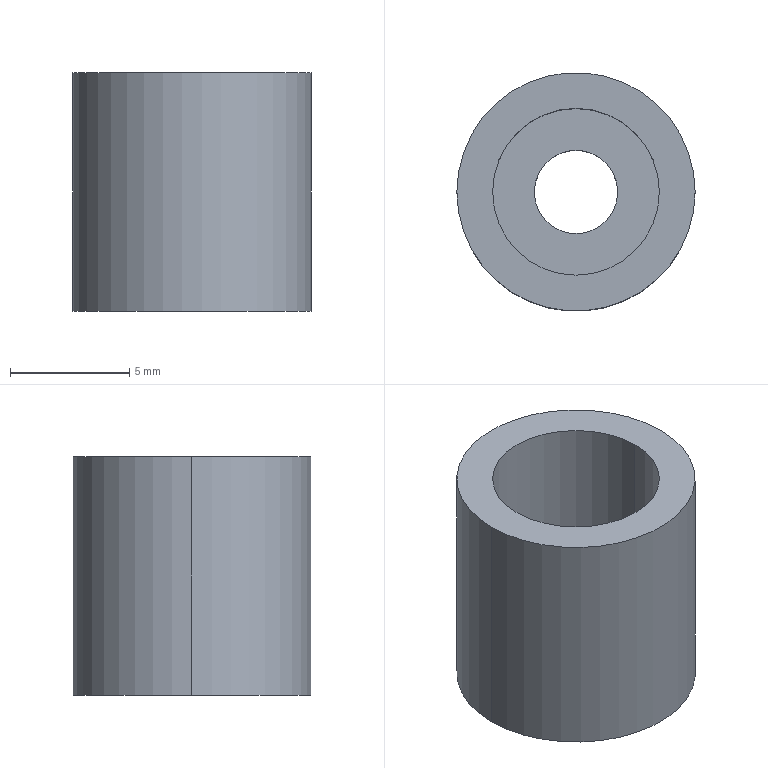Part | NX | features BREP 1 | 1 solid | 9 faces | box 10 x 10 x 10 mm | volume 544.87 mm3 | cylinder 6 | plane 3 | commonest cylinder face diameters 3.5 x2 7 x2 10 x2
STEP:
#1=CARTESIAN_POINT('',(-3.5,0.,10.));
#2=VERTEX_POINT('',#1);
#3=CARTESIAN_POINT('',(-3.5,0.,5.));
#4=VERTEX_POINT('',#3);
#5=CARTESIAN_POINT('',(-3.5,0.,10.));
#6=DIRECTION('',(0.,0.,1.));
#7=VECTOR('',#6,1000.);
#8=LINE('',#5,#7);
#9=EDGE_CURVE('',#2,#4,#8,.F.);
#10=ORIENTED_EDGE('',*,*,#9,.T.);
#11=CARTESIAN_POINT('',(3.5,0.,5.));
#12=VERTEX_POINT('',#11);
#13=CARTESIAN_POINT('',(0.,0.,5.));
#14=DIRECTION('',(0.,0.,1.));
#15=DIRECTION('',(1.,0.,0.));
#16=AXIS2_PLACEMENT_3D('',#13,#14,#15);
#17=CIRCLE('',#16,3.5);
#18=EDGE_CURVE('',#12,#4,#17,.T.);
#19=ORIENTED_EDGE('',*,*,#18,.F.);
#20=CARTESIAN_POINT('',(3.5,0.,10.));
#21=VERTEX_POINT('',#20);
#22=CARTESIAN_POINT('',(3.5,0.,10.));
#23=DIRECTION('',(0.,0.,1.));
#24=VECTOR('',#23,1000.);
#25=LINE('',#22,#24);
#26=EDGE_CURVE('',#21,#12,#25,.F.);
#27=ORIENTED_EDGE('',*,*,#26,.F.);
#28=CARTESIAN_POINT('',(0.,0.,10.));
#29=DIRECTION('',(0.,0.,1.));
#30=DIRECTION('',(1.,0.,0.));
#31=AXIS2_PLACEMENT_3D('',#28,#29,#30);
#32=CIRCLE('',#31,3.5);
#33=EDGE_CURVE('',#21,#2,#32,.T.);
#34=ORIENTED_EDGE('',*,*,#33,.T.);
#35=EDGE_LOOP('',(#10,#19,#27,#34));
#36=FACE_BOUND('',#35,.T.);
#37=CARTESIAN_POINT('',(0.,0.,10.));
#38=DIRECTION('',(0.,0.,1.));
#39=DIRECTION('',(1.,0.,0.));
#40=AXIS2_PLACEMENT_3D('',#37,#38,#39);
#41=CYLINDRICAL_SURFACE('',#40,3.5);
#42=ADVANCED_FACE('',(#36),#41,.F.);
#43=ORIENTED_EDGE('',*,*,#18,.T.);
#44=CARTESIAN_POINT('',(0.,0.,5.));
#45=DIRECTION('',(0.,0.,1.));
#46=DIRECTION('',(1.,0.,0.));
#47=AXIS2_PLACEMENT_3D('',#44,#45,#46);
#48=CIRCLE('',#47,3.5);
#49=EDGE_CURVE('',#4,#12,#48,.T.);
#50=ORIENTED_EDGE('',*,*,#49,.T.);
#51=EDGE_LOOP('',(#43,#50));
#52=FACE_BOUND('',#51,.T.);
#53=CARTESIAN_POINT('',(1.75,0.,5.));
#54=VERTEX_POINT('',#53);
#55=CARTESIAN_POINT('',(-1.75,0.,5.));
#56=VERTEX_POINT('',#55);
#57=CARTESIAN_POINT('',(0.,0.,5.));
#58=DIRECTION('',(0.,0.,1.));
#59=DIRECTION('',(1.,0.,0.));
#60=AXIS2_PLACEMENT_3D('',#57,#58,#59);
#61=CIRCLE('',#60,1.75);
#62=EDGE_CURVE('',#54,#56,#61,.T.);
#63=ORIENTED_EDGE('',*,*,#62,.F.);
#64=CARTESIAN_POINT('',(0.,0.,5.));
#65=DIRECTION('',(0.,0.,1.));
#66=DIRECTION('',(1.,0.,0.));
#67=AXIS2_PLACEMENT_3D('',#64,#65,#66);
#68=CIRCLE('',#67,1.75);
#69=EDGE_CURVE('',#56,#54,#68,.T.);
#70=ORIENTED_EDGE('',*,*,#69,.F.);
#71=EDGE_LOOP('',(#63,#70));
#72=FACE_BOUND('',#71,.T.);
#73=CARTESIAN_POINT('',(1.75,0.,5.));
#74=DIRECTION('',(0.,0.,-1.));
#75=DIRECTION('',(-1.,0.,0.));
#76=AXIS2_PLACEMENT_3D('',#73,#74,#75);
#77=PLANE('',#76);
#78=ADVANCED_FACE('',(#52,#72),#77,.F.);
#79=CARTESIAN_POINT('',(-1.75,0.,0.));
#80=VERTEX_POINT('',#79);
#81=CARTESIAN_POINT('',(-1.75,0.,10.));
#82=DIRECTION('',(0.,0.,1.));
#83=VECTOR('',#82,1000.);
#84=LINE('',#81,#83);
#85=EDGE_CURVE('',#56,#80,#84,.F.);
#86=ORIENTED_EDGE('',*,*,#85,.T.);
#87=CARTESIAN_POINT('',(1.75,0.,0.));
#88=VERTEX_POINT('',#87);
#89=CARTESIAN_POINT('',(0.,0.,0.));
#90=DIRECTION('',(0.,0.,1.));
#91=DIRECTION('',(1.,0.,0.));
#92=AXIS2_PLACEMENT_3D('',#89,#90,#91);
#93=CIRCLE('',#92,1.75);
#94=EDGE_CURVE('',#88,#80,#93,.T.);
#95=ORIENTED_EDGE('',*,*,#94,.F.);
#96=CARTESIAN_POINT('',(1.75,0.,10.));
#97=DIRECTION('',(0.,0.,1.));
#98=VECTOR('',#97,1000.);
#99=LINE('',#96,#98);
#100=EDGE_CURVE('',#54,#88,#99,.F.);
#101=ORIENTED_EDGE('',*,*,#100,.F.);
#102=ORIENTED_EDGE('',*,*,#62,.T.);
#103=EDGE_LOOP('',(#86,#95,#101,#102));
#104=FACE_BOUND('',#103,.T.);
#105=CARTESIAN_POINT('',(0.,0.,10.));
#106=DIRECTION('',(0.,0.,1.));
#107=DIRECTION('',(1.,0.,0.));
#108=AXIS2_PLACEMENT_3D('',#105,#106,#107);
#109=CYLINDRICAL_SURFACE('',#108,1.75);
#110=ADVANCED_FACE('',(#104),#109,.F.);
#111=CARTESIAN_POINT('',(-5.,0.,0.));
#112=VERTEX_POINT('',#111);
#113=CARTESIAN_POINT('',(5.,0.,0.));
#114=VERTEX_POINT('',#113);
#115=CARTESIAN_POINT('',(0.,0.,0.));
#116=DIRECTION('',(0.,0.,1.));
#117=DIRECTION('',(1.,0.,0.));
#118=AXIS2_PLACEMENT_3D('',#115,#116,#117);
#119=CIRCLE('',#118,5.);
#120=EDGE_CURVE('',#112,#114,#119,.T.);
#121=ORIENTED_EDGE('',*,*,#120,.F.);
#122=CARTESIAN_POINT('',(0.,0.,0.));
#123=DIRECTION('',(0.,0.,1.));
#124=DIRECTION('',(1.,0.,0.));
#125=AXIS2_PLACEMENT_3D('',#122,#123,#124);
#126=CIRCLE('',#125,5.);
#127=EDGE_CURVE('',#114,#112,#126,.T.);
#128=ORIENTED_EDGE('',*,*,#127,.F.);
#129=EDGE_LOOP('',(#121,#128));
#130=FACE_BOUND('',#129,.T.);
#131=ORIENTED_EDGE('',*,*,#94,.T.);
#132=CARTESIAN_POINT('',(0.,0.,0.));
#133=DIRECTION('',(0.,0.,1.));
#134=DIRECTION('',(1.,0.,0.));
#135=AXIS2_PLACEMENT_3D('',#132,#133,#134);
#136=CIRCLE('',#135,1.75);
#137=EDGE_CURVE('',#80,#88,#136,.T.);
#138=ORIENTED_EDGE('',*,*,#137,.T.);
#139=EDGE_LOOP('',(#131,#138));
#140=FACE_BOUND('',#139,.T.);
#141=CARTESIAN_POINT('',(0.,0.,0.));
#142=DIRECTION('',(0.,0.,1.));
#143=DIRECTION('',(1.,0.,0.));
#144=AXIS2_PLACEMENT_3D('',#141,#142,#143);
#145=PLANE('',#144);
#146=ADVANCED_FACE('',(#130,#140),#145,.F.);
#147=CARTESIAN_POINT('',(-5.,0.,10.));
#148=VERTEX_POINT('',#147);
#149=CARTESIAN_POINT('',(5.,0.,10.));
#150=VERTEX_POINT('',#149);
#151=CARTESIAN_POINT('',(0.,0.,10.));
#152=DIRECTION('',(0.,0.,1.));
#153=DIRECTION('',(1.,0.,0.));
#154=AXIS2_PLACEMENT_3D('',#151,#152,#153);
#155=CIRCLE('',#154,5.);
#156=EDGE_CURVE('',#148,#150,#155,.T.);
#157=ORIENTED_EDGE('',*,*,#156,.T.);
#158=CARTESIAN_POINT('',(0.,0.,10.));
#159=DIRECTION('',(0.,0.,1.));
#160=DIRECTION('',(1.,0.,0.));
#161=AXIS2_PLACEMENT_3D('',#158,#159,#160);
#162=CIRCLE('',#161,5.);
#163=EDGE_CURVE('',#150,#148,#162,.T.);
#164=ORIENTED_EDGE('',*,*,#163,.T.);
#165=EDGE_LOOP('',(#157,#164));
#166=FACE_BOUND('',#165,.T.);
#167=ORIENTED_EDGE('',*,*,#33,.F.);
#168=CARTESIAN_POINT('',(0.,0.,10.));
#169=DIRECTION('',(0.,0.,1.));
#170=DIRECTION('',(1.,0.,0.));
#171=AXIS2_PLACEMENT_3D('',#168,#169,#170);
#172=CIRCLE('',#171,3.5);
#173=EDGE_CURVE('',#2,#21,#172,.T.);
#174=ORIENTED_EDGE('',*,*,#173,.F.);
#175=EDGE_LOOP('',(#167,#174));
#176=FACE_BOUND('',#175,.T.);
#177=CARTESIAN_POINT('',(0.,0.,10.));
#178=DIRECTION('',(0.,0.,1.));
#179=DIRECTION('',(1.,0.,0.));
#180=AXIS2_PLACEMENT_3D('',#177,#178,#179);
#181=PLANE('',#180);
#182=ADVANCED_FACE('',(#166,#176),#181,.T.);
#183=CARTESIAN_POINT('',(5.,0.,10.));
#184=DIRECTION('',(0.,0.,-1.));
#185=VECTOR('',#184,1000.);
#186=LINE('',#183,#185);
#187=EDGE_CURVE('',#150,#114,#186,.T.);
#188=ORIENTED_EDGE('',*,*,#187,.F.);
#189=ORIENTED_EDGE('',*,*,#156,.F.);
#190=CARTESIAN_POINT('',(-5.,0.,10.));
#191=DIRECTION('',(0.,0.,-1.));
#192=VECTOR('',#191,1000.);
#193=LINE('',#190,#192);
#194=EDGE_CURVE('',#148,#112,#193,.T.);
#195=ORIENTED_EDGE('',*,*,#194,.T.);
#196=ORIENTED_EDGE('',*,*,#120,.T.);
#197=EDGE_LOOP('',(#188,#189,#195,#196));
#198=FACE_BOUND('',#197,.T.);
#199=CARTESIAN_POINT('',(0.,0.,10.));
#200=DIRECTION('',(0.,0.,-1.));
#201=DIRECTION('',(-1.,0.,0.));
#202=AXIS2_PLACEMENT_3D('',#199,#200,#201);
#203=CYLINDRICAL_SURFACE('',#202,5.);
#204=ADVANCED_FACE('',(#198),#203,.T.);
#205=ORIENTED_EDGE('',*,*,#163,.F.);
#206=ORIENTED_EDGE('',*,*,#187,.T.);
#207=ORIENTED_EDGE('',*,*,#127,.T.);
#208=ORIENTED_EDGE('',*,*,#194,.F.);
#209=EDGE_LOOP('',(#205,#206,#207,#208));
#210=FACE_BOUND('',#209,.T.);
#211=CARTESIAN_POINT('',(0.,0.,10.));
#212=DIRECTION('',(0.,0.,-1.));
#213=DIRECTION('',(-1.,0.,0.));
#214=AXIS2_PLACEMENT_3D('',#211,#212,#213);
#215=CYLINDRICAL_SURFACE('',#214,5.);
#216=ADVANCED_FACE('',(#210),#215,.T.);
#217=ORIENTED_EDGE('',*,*,#137,.F.);
#218=ORIENTED_EDGE('',*,*,#85,.F.);
#219=ORIENTED_EDGE('',*,*,#69,.T.);
#220=ORIENTED_EDGE('',*,*,#100,.T.);
#221=EDGE_LOOP('',(#217,#218,#219,#220));
#222=FACE_BOUND('',#221,.T.);
#223=CARTESIAN_POINT('',(0.,0.,10.));
#224=DIRECTION('',(0.,0.,1.));
#225=DIRECTION('',(1.,0.,0.));
#226=AXIS2_PLACEMENT_3D('',#223,#224,#225);
#227=CYLINDRICAL_SURFACE('',#226,1.75);
#228=ADVANCED_FACE('',(#222),#227,.F.);
#229=ORIENTED_EDGE('',*,*,#49,.F.);
#230=ORIENTED_EDGE('',*,*,#9,.F.);
#231=ORIENTED_EDGE('',*,*,#173,.T.);
#232=ORIENTED_EDGE('',*,*,#26,.T.);
#233=EDGE_LOOP('',(#229,#230,#231,#232));
#234=FACE_BOUND('',#233,.T.);
#235=CARTESIAN_POINT('',(0.,0.,10.));
#236=DIRECTION('',(0.,0.,1.));
#237=DIRECTION('',(1.,0.,0.));
#238=AXIS2_PLACEMENT_3D('',#235,#236,#237);
#239=CYLINDRICAL_SURFACE('',#238,3.5);
#240=ADVANCED_FACE('',(#234),#239,.F.);
#241=CLOSED_SHELL('',(#42,#78,#110,#146,#182,#204,#216,#228,#240));
#242=MANIFOLD_SOLID_BREP('',#241);
#243=(LENGTH_UNIT()NAMED_UNIT(*)SI_UNIT(.MILLI.,.METRE.));
#244=UNCERTAINTY_MEASURE_WITH_UNIT(LENGTH_MEASURE(0.00001),#243,'','');
#245=(NAMED_UNIT(*)PLANE_ANGLE_UNIT()SI_UNIT($,.RADIAN.));
#246=(NAMED_UNIT(*)SI_UNIT($,.STERADIAN.)SOLID_ANGLE_UNIT());
#247=(GEOMETRIC_REPRESENTATION_CONTEXT(3)GLOBAL_UNCERTAINTY_ASSIGNED_CONTEXT((#244))GLOBAL_UNIT_ASSIGNED_CONTEXT((#243,#245,#246))REPRESENTATION_CONTEXT('',''));
#248=ADVANCED_BREP_SHAPE_REPRESENTATION('',(#242),#247);